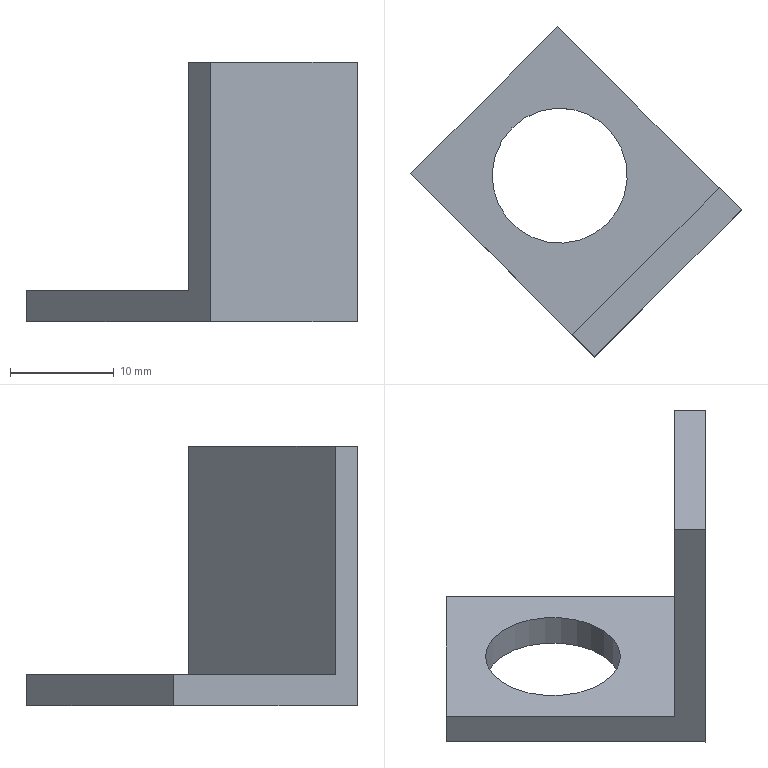Part | NX | features solid 2 | 1 solid | 9 faces | box 31.82 x 31.82 x 25 mm | volume 2422 mm3 | plane 8 | cylinder 1 | commonest cylinder face diameters 13 x1
STEP:
#1=CARTESIAN_POINT('',(-1525.048,934.698,-130.));
#2=VERTEX_POINT('',#1);
#3=CARTESIAN_POINT('',(-1539.19,920.556,-130.));
#4=VERTEX_POINT('',#3);
#5=CARTESIAN_POINT('',(-1525.048,934.698,-130.));
#6=DIRECTION('',(-0.7071,-0.7071,0.));
#7=VECTOR('',#6,1000.);
#8=LINE('',#5,#7);
#9=EDGE_CURVE('',#2,#4,#8,.T.);
#10=ORIENTED_EDGE('',*,*,#9,.T.);
#11=CARTESIAN_POINT('',(-1539.19,920.556,-127.));
#12=VERTEX_POINT('',#11);
#13=CARTESIAN_POINT('',(-1539.19,920.556,-127.));
#14=DIRECTION('',(0.,0.,-1.));
#15=VECTOR('',#14,1000.);
#16=LINE('',#13,#15);
#17=EDGE_CURVE('',#12,#4,#16,.T.);
#18=ORIENTED_EDGE('',*,*,#17,.F.);
#19=CARTESIAN_POINT('',(-1525.048,934.698,-127.));
#20=VERTEX_POINT('',#19);
#21=CARTESIAN_POINT('',(-1525.048,934.698,-127.));
#22=DIRECTION('',(-0.7071,-0.7071,0.));
#23=VECTOR('',#22,1000.);
#24=LINE('',#21,#23);
#25=EDGE_CURVE('',#20,#12,#24,.T.);
#26=ORIENTED_EDGE('',*,*,#25,.F.);
#27=CARTESIAN_POINT('',(-1525.048,934.698,-127.));
#28=DIRECTION('',(0.,0.,-1.));
#29=VECTOR('',#28,1000.);
#30=LINE('',#27,#29);
#31=EDGE_CURVE('',#20,#2,#30,.T.);
#32=ORIENTED_EDGE('',*,*,#31,.T.);
#33=EDGE_LOOP('',(#10,#18,#26,#32));
#34=FACE_BOUND('',#33,.T.);
#35=CARTESIAN_POINT('',(-1525.048,934.698,-127.));
#36=DIRECTION('',(-0.7071,0.7071,0.));
#37=DIRECTION('',(0.,0.,1.));
#38=AXIS2_PLACEMENT_3D('',#35,#36,#37);
#39=PLANE('',#38);
#40=ADVANCED_FACE('',(#34),#39,.T.);
#41=CARTESIAN_POINT('',(-1523.634,905.,-127.));
#42=VERTEX_POINT('',#41);
#43=CARTESIAN_POINT('',(-1539.19,920.556,-127.));
#44=DIRECTION('',(0.7071,-0.7071,0.));
#45=VECTOR('',#44,1000.);
#46=LINE('',#43,#45);
#47=EDGE_CURVE('',#12,#42,#46,.T.);
#48=ORIENTED_EDGE('',*,*,#47,.F.);
#49=ORIENTED_EDGE('',*,*,#17,.T.);
#50=CARTESIAN_POINT('',(-1521.512,902.879,-130.));
#51=VERTEX_POINT('',#50);
#52=CARTESIAN_POINT('',(-1539.19,920.556,-130.));
#53=DIRECTION('',(0.7071,-0.7071,0.));
#54=VECTOR('',#53,1000.);
#55=LINE('',#52,#54);
#56=EDGE_CURVE('',#4,#51,#55,.T.);
#57=ORIENTED_EDGE('',*,*,#56,.T.);
#58=CARTESIAN_POINT('',(-1521.512,902.879,-105.));
#59=VERTEX_POINT('',#58);
#60=CARTESIAN_POINT('',(-1521.512,902.879,-127.));
#61=DIRECTION('',(0.,0.,-1.));
#62=VECTOR('',#61,1000.);
#63=LINE('',#60,#62);
#64=EDGE_CURVE('',#59,#51,#63,.T.);
#65=ORIENTED_EDGE('',*,*,#64,.F.);
#66=CARTESIAN_POINT('',(-1523.634,905.,-105.));
#67=VERTEX_POINT('',#66);
#68=CARTESIAN_POINT('',(-1521.512,902.879,-105.));
#69=DIRECTION('',(-0.7071,0.7071,0.));
#70=VECTOR('',#69,1000.);
#71=LINE('',#68,#70);
#72=EDGE_CURVE('',#59,#67,#71,.T.);
#73=ORIENTED_EDGE('',*,*,#72,.T.);
#74=CARTESIAN_POINT('',(-1523.634,905.,-130.));
#75=DIRECTION('',(0.,0.,1.));
#76=VECTOR('',#75,1000.);
#77=LINE('',#74,#76);
#78=EDGE_CURVE('',#42,#67,#77,.T.);
#79=ORIENTED_EDGE('',*,*,#78,.F.);
#80=EDGE_LOOP('',(#48,#49,#57,#65,#73,#79));
#81=FACE_BOUND('',#80,.T.);
#82=CARTESIAN_POINT('',(-1539.19,920.556,-127.));
#83=DIRECTION('',(-0.7071,-0.7071,0.));
#84=DIRECTION('',(0.,0.,1.));
#85=AXIS2_PLACEMENT_3D('',#82,#83,#84);
#86=PLANE('',#85);
#87=ADVANCED_FACE('',(#81),#86,.T.);
#88=CARTESIAN_POINT('',(-1507.37,917.021,-130.));
#89=VERTEX_POINT('',#88);
#90=CARTESIAN_POINT('',(-1521.512,902.879,-130.));
#91=DIRECTION('',(0.7071,0.7071,0.));
#92=VECTOR('',#91,1000.);
#93=LINE('',#90,#92);
#94=EDGE_CURVE('',#51,#89,#93,.T.);
#95=ORIENTED_EDGE('',*,*,#94,.T.);
#96=CARTESIAN_POINT('',(-1507.37,917.021,-105.));
#97=VERTEX_POINT('',#96);
#98=CARTESIAN_POINT('',(-1507.37,917.021,-127.));
#99=DIRECTION('',(0.,0.,-1.));
#100=VECTOR('',#99,1000.);
#101=LINE('',#98,#100);
#102=EDGE_CURVE('',#97,#89,#101,.T.);
#103=ORIENTED_EDGE('',*,*,#102,.F.);
#104=CARTESIAN_POINT('',(-1521.512,902.879,-105.));
#105=DIRECTION('',(0.7071,0.7071,0.));
#106=VECTOR('',#105,1000.);
#107=LINE('',#104,#106);
#108=EDGE_CURVE('',#59,#97,#107,.T.);
#109=ORIENTED_EDGE('',*,*,#108,.F.);
#110=ORIENTED_EDGE('',*,*,#64,.T.);
#111=EDGE_LOOP('',(#95,#103,#109,#110));
#112=FACE_BOUND('',#111,.T.);
#113=CARTESIAN_POINT('',(-1521.512,902.879,-127.));
#114=DIRECTION('',(0.7071,-0.7071,0.));
#115=DIRECTION('',(0.,0.,-1.));
#116=AXIS2_PLACEMENT_3D('',#113,#114,#115);
#117=PLANE('',#116);
#118=ADVANCED_FACE('',(#112),#117,.T.);
#119=ORIENTED_EDGE('',*,*,#31,.F.);
#120=CARTESIAN_POINT('',(-1509.492,919.142,-127.));
#121=VERTEX_POINT('',#120);
#122=CARTESIAN_POINT('',(-1507.37,917.021,-127.));
#123=DIRECTION('',(-0.7071,0.7071,0.));
#124=VECTOR('',#123,1000.);
#125=LINE('',#122,#124);
#126=EDGE_CURVE('',#121,#20,#125,.T.);
#127=ORIENTED_EDGE('',*,*,#126,.F.);
#128=CARTESIAN_POINT('',(-1509.492,919.142,-105.));
#129=VERTEX_POINT('',#128);
#130=CARTESIAN_POINT('',(-1509.492,919.142,-130.));
#131=DIRECTION('',(0.,0.,1.));
#132=VECTOR('',#131,1000.);
#133=LINE('',#130,#132);
#134=EDGE_CURVE('',#121,#129,#133,.T.);
#135=ORIENTED_EDGE('',*,*,#134,.T.);
#136=CARTESIAN_POINT('',(-1507.37,917.021,-105.));
#137=DIRECTION('',(-0.7071,0.7071,0.));
#138=VECTOR('',#137,1000.);
#139=LINE('',#136,#138);
#140=EDGE_CURVE('',#97,#129,#139,.T.);
#141=ORIENTED_EDGE('',*,*,#140,.F.);
#142=ORIENTED_EDGE('',*,*,#102,.T.);
#143=CARTESIAN_POINT('',(-1507.37,917.021,-130.));
#144=DIRECTION('',(-0.7071,0.7071,0.));
#145=VECTOR('',#144,1000.);
#146=LINE('',#143,#145);
#147=EDGE_CURVE('',#89,#2,#146,.T.);
#148=ORIENTED_EDGE('',*,*,#147,.T.);
#149=EDGE_LOOP('',(#119,#127,#135,#141,#142,#148));
#150=FACE_BOUND('',#149,.T.);
#151=CARTESIAN_POINT('',(-1507.37,917.021,-127.));
#152=DIRECTION('',(0.7071,0.7071,0.));
#153=DIRECTION('',(0.7071,-0.7071,0.));
#154=AXIS2_PLACEMENT_3D('',#151,#152,#153);
#155=PLANE('',#154);
#156=ADVANCED_FACE('',(#150),#155,.T.);
#157=CARTESIAN_POINT('',(-1520.252,915.761,-127.));
#158=VERTEX_POINT('',#157);
#159=CARTESIAN_POINT('',(-1524.848,920.357,-127.));
#160=DIRECTION('',(0.,0.,-1.));
#161=DIRECTION('',(0.7071,-0.7071,0.));
#162=AXIS2_PLACEMENT_3D('',#159,#160,#161);
#163=CIRCLE('',#162,6.5);
#164=EDGE_CURVE('',#158,#158,#163,.T.);
#165=ORIENTED_EDGE('',*,*,#164,.F.);
#166=EDGE_LOOP('',(#165));
#167=FACE_BOUND('',#166,.T.);
#168=CARTESIAN_POINT('',(-1520.252,915.761,-130.));
#169=VERTEX_POINT('',#168);
#170=CARTESIAN_POINT('',(-1524.848,920.357,-130.));
#171=DIRECTION('',(0.,0.,-1.));
#172=DIRECTION('',(0.7071,-0.7071,0.));
#173=AXIS2_PLACEMENT_3D('',#170,#171,#172);
#174=CIRCLE('',#173,6.5);
#175=EDGE_CURVE('',#169,#169,#174,.T.);
#176=ORIENTED_EDGE('',*,*,#175,.T.);
#177=EDGE_LOOP('',(#176));
#178=FACE_BOUND('',#177,.T.);
#179=CARTESIAN_POINT('',(-1524.848,920.357,-127.));
#180=DIRECTION('',(0.,0.,-1.));
#181=DIRECTION('',(-0.7071,0.7071,0.));
#182=AXIS2_PLACEMENT_3D('',#179,#180,#181);
#183=CYLINDRICAL_SURFACE('',#182,6.5);
#184=ADVANCED_FACE('',(#167,#178),#183,.F.);
#185=ORIENTED_EDGE('',*,*,#126,.T.);
#186=ORIENTED_EDGE('',*,*,#25,.T.);
#187=ORIENTED_EDGE('',*,*,#47,.T.);
#188=CARTESIAN_POINT('',(-1523.634,905.,-127.));
#189=DIRECTION('',(-0.7071,-0.7071,0.));
#190=VECTOR('',#189,1000.);
#191=LINE('',#188,#190);
#192=EDGE_CURVE('',#121,#42,#191,.T.);
#193=ORIENTED_EDGE('',*,*,#192,.F.);
#194=EDGE_LOOP('',(#185,#186,#187,#193));
#195=FACE_BOUND('',#194,.T.);
#196=ORIENTED_EDGE('',*,*,#164,.T.);
#197=EDGE_LOOP('',(#196));
#198=FACE_BOUND('',#197,.T.);
#199=CARTESIAN_POINT('',(-1539.19,920.556,-127.));
#200=DIRECTION('',(0.,0.,-1.));
#201=DIRECTION('',(-0.7071,0.7071,0.));
#202=AXIS2_PLACEMENT_3D('',#199,#200,#201);
#203=PLANE('',#202);
#204=ADVANCED_FACE('',(#195,#198),#203,.F.);
#205=ORIENTED_EDGE('',*,*,#56,.F.);
#206=ORIENTED_EDGE('',*,*,#9,.F.);
#207=ORIENTED_EDGE('',*,*,#147,.F.);
#208=ORIENTED_EDGE('',*,*,#94,.F.);
#209=EDGE_LOOP('',(#205,#206,#207,#208));
#210=FACE_BOUND('',#209,.T.);
#211=ORIENTED_EDGE('',*,*,#175,.F.);
#212=EDGE_LOOP('',(#211));
#213=FACE_BOUND('',#212,.T.);
#214=CARTESIAN_POINT('',(-1539.19,920.556,-130.));
#215=DIRECTION('',(0.,0.,-1.));
#216=DIRECTION('',(-0.7071,0.7071,0.));
#217=AXIS2_PLACEMENT_3D('',#214,#215,#216);
#218=PLANE('',#217);
#219=ADVANCED_FACE('',(#210,#213),#218,.T.);
#220=ORIENTED_EDGE('',*,*,#192,.T.);
#221=ORIENTED_EDGE('',*,*,#78,.T.);
#222=CARTESIAN_POINT('',(-1523.634,905.,-105.));
#223=DIRECTION('',(-0.7071,-0.7071,0.));
#224=VECTOR('',#223,1000.);
#225=LINE('',#222,#224);
#226=EDGE_CURVE('',#67,#129,#225,.F.);
#227=ORIENTED_EDGE('',*,*,#226,.T.);
#228=ORIENTED_EDGE('',*,*,#134,.F.);
#229=EDGE_LOOP('',(#220,#221,#227,#228));
#230=FACE_BOUND('',#229,.T.);
#231=CARTESIAN_POINT('',(-1523.634,905.,-130.));
#232=DIRECTION('',(-0.7071,0.7071,0.));
#233=DIRECTION('',(0.,0.,1.));
#234=AXIS2_PLACEMENT_3D('',#231,#232,#233);
#235=PLANE('',#234);
#236=ADVANCED_FACE('',(#230),#235,.T.);
#237=ORIENTED_EDGE('',*,*,#140,.T.);
#238=ORIENTED_EDGE('',*,*,#226,.F.);
#239=ORIENTED_EDGE('',*,*,#72,.F.);
#240=ORIENTED_EDGE('',*,*,#108,.T.);
#241=EDGE_LOOP('',(#237,#238,#239,#240));
#242=FACE_BOUND('',#241,.T.);
#243=CARTESIAN_POINT('',(-1521.512,902.879,-105.));
#244=DIRECTION('',(0.,0.,-1.));
#245=DIRECTION('',(0.7071,0.7071,0.));
#246=AXIS2_PLACEMENT_3D('',#243,#244,#245);
#247=PLANE('',#246);
#248=ADVANCED_FACE('',(#242),#247,.F.);
#249=CLOSED_SHELL('',(#40,#87,#118,#156,#184,#204,#219,#236,#248));
#250=MANIFOLD_SOLID_BREP('',#249);
#251=(LENGTH_UNIT()NAMED_UNIT(*)SI_UNIT(.MILLI.,.METRE.));
#252=UNCERTAINTY_MEASURE_WITH_UNIT(LENGTH_MEASURE(0.00001),#251,'','');
#253=(NAMED_UNIT(*)PLANE_ANGLE_UNIT()SI_UNIT($,.RADIAN.));
#254=(NAMED_UNIT(*)SI_UNIT($,.STERADIAN.)SOLID_ANGLE_UNIT());
#255=(GEOMETRIC_REPRESENTATION_CONTEXT(3)GLOBAL_UNCERTAINTY_ASSIGNED_CONTEXT((#252))GLOBAL_UNIT_ASSIGNED_CONTEXT((#251,#253,#254))REPRESENTATION_CONTEXT('',''));
#256=ADVANCED_BREP_SHAPE_REPRESENTATION('',(#250),#255);